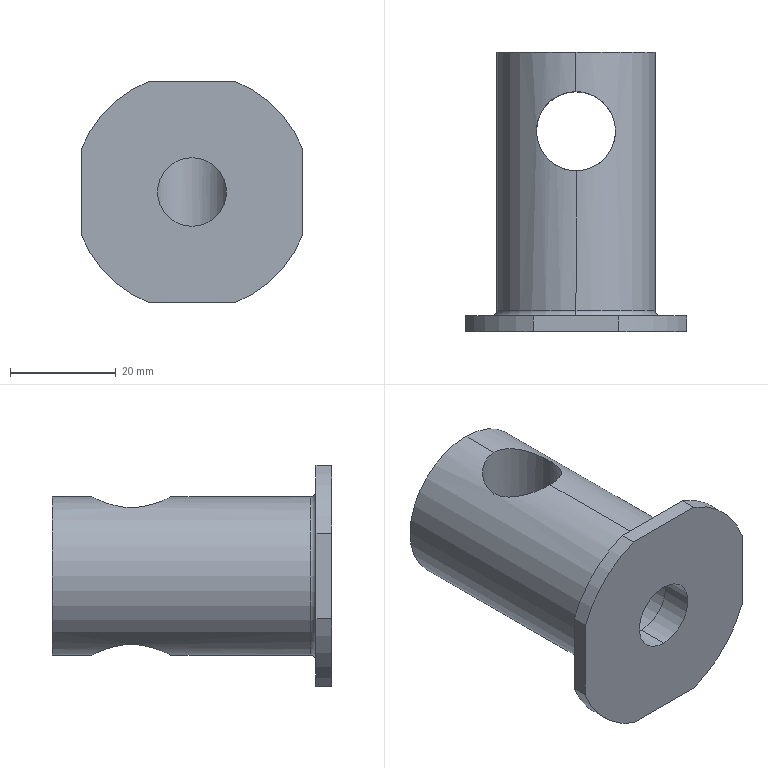Part | SolidWorks | features ICE 8, Fillet 2, MoveFace 1, Revolution 1 | 1 solid | 22 faces | box 42 x 53 x 42 mm | volume 30095 mm3 | cylinder 12 | plane 8 | torus 2 | commonest cylinder face diameters 45 x4 13 x2 14 x2 15 x2 30 x2
STEP:
#1=CARTESIAN_POINT('',(0.,31.,7.));
#2=VERTEX_POINT('',#1);
#3=CARTESIAN_POINT('',(0.,31.,-7.));
#4=VERTEX_POINT('',#3);
#5=CARTESIAN_POINT('',(0.,31.,7.));
#6=CARTESIAN_POINT('',(0.5148,31.,7.));
#7=CARTESIAN_POINT('',(1.015,31.052,6.944));
#8=CARTESIAN_POINT('',(1.746,31.202,6.783));
#9=CARTESIAN_POINT('',(1.988,31.264,6.716));
#10=CARTESIAN_POINT('',(2.452,31.408,6.561));
#11=CARTESIAN_POINT('',(2.676,31.49,6.473));
#12=CARTESIAN_POINT('',(3.325,31.761,6.178));
#13=CARTESIAN_POINT('',(3.73,31.979,5.941));
#14=CARTESIAN_POINT('',(4.457,32.452,5.416));
#15=CARTESIAN_POINT('',(4.784,32.71,5.128));
#16=CARTESIAN_POINT('',(5.228,33.118,4.66));
#17=CARTESIAN_POINT('',(5.368,33.259,4.498));
#18=CARTESIAN_POINT('',(5.63,33.541,4.165));
#19=CARTESIAN_POINT('',(5.752,33.684,3.994));
#20=CARTESIAN_POINT('',(6.094,34.112,3.47));
#21=CARTESIAN_POINT('',(6.288,34.4,3.104));
#22=CARTESIAN_POINT('',(6.617,34.955,2.322));
#23=CARTESIAN_POINT('',(6.752,35.227,1.904));
#24=CARTESIAN_POINT('',(6.896,35.549,1.224));
#25=CARTESIAN_POINT('',(6.935,35.643,0.9854));
#26=CARTESIAN_POINT('',(6.974,35.74,0.6181));
#27=CARTESIAN_POINT('',(6.984,35.765,0.494));
#28=CARTESIAN_POINT('',(6.997,35.8,0.2415));
#29=CARTESIAN_POINT('',(7.,35.808,0.112));
#30=CARTESIAN_POINT('',(6.999,35.806,-0.2717));
#31=CARTESIAN_POINT('',(6.985,35.767,-0.5222));
#32=CARTESIAN_POINT('',(6.93,35.632,-1.015));
#33=CARTESIAN_POINT('',(6.891,35.538,-1.249));
#34=CARTESIAN_POINT('',(6.795,35.323,-1.699));
#35=CARTESIAN_POINT('',(6.737,35.2,-1.915));
#36=CARTESIAN_POINT('',(6.603,34.94,-2.334));
#37=CARTESIAN_POINT('',(6.528,34.804,-2.535));
#38=CARTESIAN_POINT('',(6.28,34.388,-3.12));
#39=CARTESIAN_POINT('',(6.085,34.1,-3.486));
#40=CARTESIAN_POINT('',(5.626,33.527,-4.186));
#41=CARTESIAN_POINT('',(5.362,33.241,-4.52));
#42=CARTESIAN_POINT('',(4.774,32.702,-5.138));
#43=CARTESIAN_POINT('',(4.449,32.446,-5.423));
#44=CARTESIAN_POINT('',(3.905,32.093,-5.814));
#45=CARTESIAN_POINT('',(3.715,31.981,-5.937));
#46=CARTESIAN_POINT('',(3.313,31.767,-6.171));
#47=CARTESIAN_POINT('',(3.103,31.668,-6.279));
#48=CARTESIAN_POINT('',(2.671,31.488,-6.475));
#49=CARTESIAN_POINT('',(2.447,31.406,-6.563));
#50=CARTESIAN_POINT('',(1.985,31.263,-6.717));
#51=CARTESIAN_POINT('',(1.744,31.201,-6.784));
#52=CARTESIAN_POINT('',(1.01,31.051,-6.945));
#53=CARTESIAN_POINT('',(0.5101,31.,-7.));
#54=CARTESIAN_POINT('',(0.,31.,-7.));
#55=B_SPLINE_CURVE_WITH_KNOTS('',3,(#5,#6,#7,#8,#9,#10,#11,#12,#13,#14,#15,#16,#17,#18,#19,#20,#21,#22,#23,#24,#25,#26,#27,#28,#29,#30,#31,#32,#33,#34,#35,#36,#37,#38,#39,#40,#41,#42,#43,#44,#45,#46,#47,#48,#49,#50,#51,#52,#53,#54),.UNSPECIFIED.,.F.,.F.,(4,2,2,2,2,2,2,2,2,2,2,2,2,2,2,2,2,2,2,2,2,2,2,2,4),(0.,0.001518,0.002277,0.003036,0.004554,0.006073,0.006832,0.007591,0.009109,0.01063,0.01139,0.01177,0.01215,0.0129,0.01366,0.01442,0.01518,0.0167,0.01822,0.01974,0.02049,0.02125,0.02201,0.02277,0.02429),.UNSPECIFIED.);
#56=EDGE_CURVE('',#2,#4,#55,.T.);
#57=ORIENTED_EDGE('',*,*,#56,.F.);
#58=CARTESIAN_POINT('',(0.,31.,-7.));
#59=CARTESIAN_POINT('',(-0.2549,31.,-7.));
#60=CARTESIAN_POINT('',(-0.5127,31.013,-6.986));
#61=CARTESIAN_POINT('',(-1.015,31.065,-6.931));
#62=CARTESIAN_POINT('',(-1.263,31.103,-6.89));
#63=CARTESIAN_POINT('',(-1.75,31.203,-6.782));
#64=CARTESIAN_POINT('',(-1.991,31.265,-6.715));
#65=CARTESIAN_POINT('',(-2.455,31.409,-6.56));
#66=CARTESIAN_POINT('',(-2.679,31.491,-6.471));
#67=CARTESIAN_POINT('',(-3.328,31.763,-6.177));
#68=CARTESIAN_POINT('',(-3.733,31.98,-5.939));
#69=CARTESIAN_POINT('',(-4.459,32.454,-5.414));
#70=CARTESIAN_POINT('',(-4.786,32.711,-5.127));
#71=CARTESIAN_POINT('',(-5.229,33.12,-4.659));
#72=CARTESIAN_POINT('',(-5.369,33.26,-4.496));
#73=CARTESIAN_POINT('',(-5.631,33.543,-4.163));
#74=CARTESIAN_POINT('',(-5.753,33.685,-3.993));
#75=CARTESIAN_POINT('',(-6.094,34.113,-3.469));
#76=CARTESIAN_POINT('',(-6.289,34.401,-3.103));
#77=CARTESIAN_POINT('',(-6.617,34.956,-2.321));
#78=CARTESIAN_POINT('',(-6.752,35.227,-1.903));
#79=CARTESIAN_POINT('',(-6.896,35.549,-1.224));
#80=CARTESIAN_POINT('',(-6.935,35.643,-0.9852));
#81=CARTESIAN_POINT('',(-6.974,35.74,-0.6182));
#82=CARTESIAN_POINT('',(-6.984,35.765,-0.4941));
#83=CARTESIAN_POINT('',(-6.997,35.799,-0.2417));
#84=CARTESIAN_POINT('',(-7.,35.808,-0.1122));
#85=CARTESIAN_POINT('',(-6.999,35.806,0.2711));
#86=CARTESIAN_POINT('',(-6.985,35.768,0.5215));
#87=CARTESIAN_POINT('',(-6.931,35.633,1.014));
#88=CARTESIAN_POINT('',(-6.892,35.539,1.248));
#89=CARTESIAN_POINT('',(-6.795,35.323,1.697));
#90=CARTESIAN_POINT('',(-6.737,35.201,1.914));
#91=CARTESIAN_POINT('',(-6.603,34.941,2.333));
#92=CARTESIAN_POINT('',(-6.529,34.805,2.534));
#93=CARTESIAN_POINT('',(-6.281,34.389,3.118));
#94=CARTESIAN_POINT('',(-6.086,34.101,3.484));
#95=CARTESIAN_POINT('',(-5.628,33.529,4.184));
#96=CARTESIAN_POINT('',(-5.364,33.243,4.518));
#97=CARTESIAN_POINT('',(-4.776,32.704,5.135));
#98=CARTESIAN_POINT('',(-4.452,32.449,5.421));
#99=CARTESIAN_POINT('',(-3.909,32.096,5.811));
#100=CARTESIAN_POINT('',(-3.719,31.983,5.935));
#101=CARTESIAN_POINT('',(-3.317,31.769,6.169));
#102=CARTESIAN_POINT('',(-3.107,31.67,6.277));
#103=CARTESIAN_POINT('',(-2.675,31.49,6.473));
#104=CARTESIAN_POINT('',(-2.452,31.408,6.561));
#105=CARTESIAN_POINT('',(-1.99,31.265,6.716));
#106=CARTESIAN_POINT('',(-1.749,31.203,6.783));
#107=CARTESIAN_POINT('',(-1.015,31.052,6.944));
#108=CARTESIAN_POINT('',(-0.5145,31.,7.));
#109=CARTESIAN_POINT('',(0.,31.,7.));
#110=B_SPLINE_CURVE_WITH_KNOTS('',3,(#58,#59,#60,#61,#62,#63,#64,#65,#66,#67,#68,#69,#70,#71,#72,#73,#74,#75,#76,#77,#78,#79,#80,#81,#82,#83,#84,#85,#86,#87,#88,#89,#90,#91,#92,#93,#94,#95,#96,#97,#98,#99,#100,#101,#102,#103,#104,#105,#106,#107,#108,#109),.UNSPECIFIED.,.F.,.F.,(4,2,2,2,2,2,2,2,2,2,2,2,2,2,2,2,2,2,2,2,2,2,2,2,2,4),(0.02429,0.02505,0.02581,0.02657,0.02732,0.02884,0.03036,0.03112,0.03188,0.03339,0.03491,0.03567,0.03605,0.03643,0.03719,0.03795,0.0387,0.03946,0.04098,0.0425,0.04401,0.04477,0.04553,0.04629,0.04705,0.04857),.UNSPECIFIED.);
#111=EDGE_CURVE('',#4,#2,#110,.T.);
#112=ORIENTED_EDGE('',*,*,#111,.F.);
#113=EDGE_LOOP('',(#57,#112));
#114=FACE_BOUND('',#113,.T.);
#115=CARTESIAN_POINT('',(0.,31.,-15.));
#116=VERTEX_POINT('',#115);
#117=CARTESIAN_POINT('',(-7.5,38.5,-12.99));
#118=VERTEX_POINT('',#117);
#119=CARTESIAN_POINT('',(0.,31.,-15.));
#120=CARTESIAN_POINT('',(-0.2495,31.,-15.));
#121=CARTESIAN_POINT('',(-0.5024,31.013,-14.994));
#122=CARTESIAN_POINT('',(-1.,31.063,-14.969));
#123=CARTESIAN_POINT('',(-1.246,31.1,-14.95));
#124=CARTESIAN_POINT('',(-1.731,31.198,-14.902));
#125=CARTESIAN_POINT('',(-1.97,31.259,-14.872));
#126=CARTESIAN_POINT('',(-2.443,31.405,-14.802));
#127=CARTESIAN_POINT('',(-2.677,31.49,-14.761));
#128=CARTESIAN_POINT('',(-3.359,31.776,-14.626));
#129=CARTESIAN_POINT('',(-3.787,32.008,-14.52));
#130=CARTESIAN_POINT('',(-4.391,32.415,-14.345));
#131=CARTESIAN_POINT('',(-4.587,32.561,-14.283));
#132=CARTESIAN_POINT('',(-4.961,32.87,-14.157));
#133=CARTESIAN_POINT('',(-5.139,33.033,-14.093));
#134=CARTESIAN_POINT('',(-5.649,33.543,-13.9));
#135=CARTESIAN_POINT('',(-5.954,33.914,-13.771));
#136=CARTESIAN_POINT('',(-6.497,34.722,-13.523));
#137=CARTESIAN_POINT('',(-6.728,35.151,-13.408));
#138=CARTESIAN_POINT('',(-7.01,35.822,-13.262));
#139=CARTESIAN_POINT('',(-7.093,36.052,-13.217));
#140=CARTESIAN_POINT('',(-7.239,36.522,-13.138));
#141=CARTESIAN_POINT('',(-7.301,36.764,-13.104));
#142=CARTESIAN_POINT('',(-7.45,37.499,-13.02));
#143=CARTESIAN_POINT('',(-7.5,37.995,-12.99));
#144=CARTESIAN_POINT('',(-7.5,38.5,-12.99));
#145=B_SPLINE_CURVE_WITH_KNOTS('',3,(#119,#120,#121,#122,#123,#124,#125,#126,#127,#128,#129,#130,#131,#132,#133,#134,#135,#136,#137,#138,#139,#140,#141,#142,#143,#144),.UNSPECIFIED.,.F.,.F.,(4,2,2,2,2,2,2,2,2,2,2,2,4),(0.01193,0.01268,0.01342,0.01417,0.01491,0.0164,0.01714,0.01789,0.01938,0.02086,0.02161,0.02235,0.02384),.UNSPECIFIED.);
#146=EDGE_CURVE('',#116,#118,#145,.T.);
#147=ORIENTED_EDGE('',*,*,#146,.T.);
#148=CARTESIAN_POINT('',(-7.5,38.5,12.99));
#149=VERTEX_POINT('',#148);
#150=CARTESIAN_POINT('',(-7.5,38.5,-15.));
#151=DIRECTION('',(0.,0.,1.));
#152=VECTOR('',#151,1000.);
#153=LINE('',#150,#152);
#154=EDGE_CURVE('',#118,#149,#153,.T.);
#155=ORIENTED_EDGE('',*,*,#154,.T.);
#156=CARTESIAN_POINT('',(0.,31.,15.));
#157=VERTEX_POINT('',#156);
#158=CARTESIAN_POINT('',(-7.5,38.5,12.99));
#159=CARTESIAN_POINT('',(-7.5,37.995,12.99));
#160=CARTESIAN_POINT('',(-7.45,37.5,13.02));
#161=CARTESIAN_POINT('',(-7.254,36.53,13.13));
#162=CARTESIAN_POINT('',(-7.106,36.05,13.212));
#163=CARTESIAN_POINT('',(-6.727,35.147,13.409));
#164=CARTESIAN_POINT('',(-6.496,34.72,13.524));
#165=CARTESIAN_POINT('',(-6.089,34.114,13.71));
#166=CARTESIAN_POINT('',(-5.943,33.918,13.774));
#167=CARTESIAN_POINT('',(-5.636,33.545,13.902));
#168=CARTESIAN_POINT('',(-5.474,33.367,13.967));
#169=CARTESIAN_POINT('',(-5.134,33.027,14.095));
#170=CARTESIAN_POINT('',(-4.955,32.865,14.159));
#171=CARTESIAN_POINT('',(-4.581,32.557,14.285));
#172=CARTESIAN_POINT('',(-4.385,32.41,14.346));
#173=CARTESIAN_POINT('',(-3.778,32.003,14.523));
#174=CARTESIAN_POINT('',(-3.351,31.772,14.628));
#175=CARTESIAN_POINT('',(-2.674,31.489,14.761));
#176=CARTESIAN_POINT('',(-2.443,31.405,14.802));
#177=CARTESIAN_POINT('',(-1.967,31.258,14.872));
#178=CARTESIAN_POINT('',(-1.724,31.197,14.903));
#179=CARTESIAN_POINT('',(-0.9934,31.05,14.975));
#180=CARTESIAN_POINT('',(-0.5001,31.,15.));
#181=CARTESIAN_POINT('',(0.,31.,15.));
#182=B_SPLINE_CURVE_WITH_KNOTS('',3,(#158,#159,#160,#161,#162,#163,#164,#165,#166,#167,#168,#169,#170,#171,#172,#173,#174,#175,#176,#177,#178,#179,#180,#181),.UNSPECIFIED.,.F.,.F.,(4,2,2,2,2,2,2,2,2,2,2,4),(0.,0.001492,0.002983,0.004475,0.00522,0.005966,0.006712,0.007458,0.008949,0.009695,0.01044,0.01193),.UNSPECIFIED.);
#183=EDGE_CURVE('',#149,#157,#182,.T.);
#184=ORIENTED_EDGE('',*,*,#183,.T.);
#185=CARTESIAN_POINT('',(7.5,38.5,12.99));
#186=VERTEX_POINT('',#185);
#187=CARTESIAN_POINT('',(0.,31.,15.));
#188=CARTESIAN_POINT('',(0.2495,31.,15.));
#189=CARTESIAN_POINT('',(0.5024,31.013,14.994));
#190=CARTESIAN_POINT('',(1.,31.063,14.969));
#191=CARTESIAN_POINT('',(1.246,31.1,14.95));
#192=CARTESIAN_POINT('',(1.731,31.198,14.902));
#193=CARTESIAN_POINT('',(1.97,31.259,14.872));
#194=CARTESIAN_POINT('',(2.443,31.405,14.802));
#195=CARTESIAN_POINT('',(2.677,31.49,14.761));
#196=CARTESIAN_POINT('',(3.359,31.776,14.626));
#197=CARTESIAN_POINT('',(3.787,32.008,14.52));
#198=CARTESIAN_POINT('',(4.391,32.415,14.345));
#199=CARTESIAN_POINT('',(4.587,32.561,14.283));
#200=CARTESIAN_POINT('',(4.961,32.87,14.157));
#201=CARTESIAN_POINT('',(5.139,33.033,14.093));
#202=CARTESIAN_POINT('',(5.649,33.543,13.9));
#203=CARTESIAN_POINT('',(5.954,33.914,13.771));
#204=CARTESIAN_POINT('',(6.497,34.722,13.523));
#205=CARTESIAN_POINT('',(6.728,35.151,13.408));
#206=CARTESIAN_POINT('',(7.01,35.822,13.262));
#207=CARTESIAN_POINT('',(7.093,36.052,13.217));
#208=CARTESIAN_POINT('',(7.239,36.522,13.138));
#209=CARTESIAN_POINT('',(7.301,36.764,13.104));
#210=CARTESIAN_POINT('',(7.45,37.499,13.02));
#211=CARTESIAN_POINT('',(7.5,37.995,12.99));
#212=CARTESIAN_POINT('',(7.5,38.5,12.99));
#213=B_SPLINE_CURVE_WITH_KNOTS('',3,(#187,#188,#189,#190,#191,#192,#193,#194,#195,#196,#197,#198,#199,#200,#201,#202,#203,#204,#205,#206,#207,#208,#209,#210,#211,#212),.UNSPECIFIED.,.F.,.F.,(4,2,2,2,2,2,2,2,2,2,2,2,4),(0.01193,0.01268,0.01342,0.01417,0.01491,0.0164,0.01714,0.01789,0.01938,0.02086,0.02161,0.02235,0.02384),.UNSPECIFIED.);
#214=EDGE_CURVE('',#157,#186,#213,.T.);
#215=ORIENTED_EDGE('',*,*,#214,.T.);
#216=CARTESIAN_POINT('',(7.5,38.5,-12.99));
#217=VERTEX_POINT('',#216);
#218=CARTESIAN_POINT('',(7.5,38.5,-15.));
#219=DIRECTION('',(0.,0.,1.));
#220=VECTOR('',#219,1000.);
#221=LINE('',#218,#220);
#222=EDGE_CURVE('',#217,#186,#221,.T.);
#223=ORIENTED_EDGE('',*,*,#222,.F.);
#224=CARTESIAN_POINT('',(7.5,38.5,-12.99));
#225=CARTESIAN_POINT('',(7.5,37.995,-12.99));
#226=CARTESIAN_POINT('',(7.45,37.5,-13.02));
#227=CARTESIAN_POINT('',(7.254,36.53,-13.13));
#228=CARTESIAN_POINT('',(7.106,36.05,-13.212));
#229=CARTESIAN_POINT('',(6.727,35.147,-13.409));
#230=CARTESIAN_POINT('',(6.496,34.72,-13.524));
#231=CARTESIAN_POINT('',(6.089,34.114,-13.71));
#232=CARTESIAN_POINT('',(5.943,33.918,-13.774));
#233=CARTESIAN_POINT('',(5.636,33.545,-13.902));
#234=CARTESIAN_POINT('',(5.474,33.367,-13.967));
#235=CARTESIAN_POINT('',(5.134,33.027,-14.095));
#236=CARTESIAN_POINT('',(4.955,32.865,-14.159));
#237=CARTESIAN_POINT('',(4.581,32.557,-14.285));
#238=CARTESIAN_POINT('',(4.385,32.41,-14.346));
#239=CARTESIAN_POINT('',(3.778,32.003,-14.523));
#240=CARTESIAN_POINT('',(3.351,31.772,-14.628));
#241=CARTESIAN_POINT('',(2.674,31.489,-14.761));
#242=CARTESIAN_POINT('',(2.443,31.405,-14.802));
#243=CARTESIAN_POINT('',(1.967,31.258,-14.872));
#244=CARTESIAN_POINT('',(1.724,31.197,-14.903));
#245=CARTESIAN_POINT('',(0.9934,31.05,-14.975));
#246=CARTESIAN_POINT('',(0.5001,31.,-15.));
#247=CARTESIAN_POINT('',(0.,31.,-15.));
#248=B_SPLINE_CURVE_WITH_KNOTS('',3,(#224,#225,#226,#227,#228,#229,#230,#231,#232,#233,#234,#235,#236,#237,#238,#239,#240,#241,#242,#243,#244,#245,#246,#247),.UNSPECIFIED.,.F.,.F.,(4,2,2,2,2,2,2,2,2,2,2,4),(0.,0.001492,0.002983,0.004475,0.00522,0.005966,0.006712,0.007458,0.008949,0.009695,0.01044,0.01193),.UNSPECIFIED.);
#249=EDGE_CURVE('',#217,#116,#248,.T.);
#250=ORIENTED_EDGE('',*,*,#249,.T.);
#251=EDGE_LOOP('',(#147,#155,#184,#215,#223,#250));
#252=FACE_OUTER_BOUND('',#251,.T.);
#253=CARTESIAN_POINT('',(0.,38.5,-15.));
#254=DIRECTION('',(0.,0.,1.));
#255=DIRECTION('',(1.,0.,0.));
#256=AXIS2_PLACEMENT_3D('',#253,#254,#255);
#257=CYLINDRICAL_SURFACE('',#256,7.5);
#258=ADVANCED_FACE('',(#114,#252),#257,.F.);
#259=CARTESIAN_POINT('',(0.,0.5,6.5));
#260=VERTEX_POINT('',#259);
#261=CARTESIAN_POINT('',(0.,0.5,-6.5));
#262=VERTEX_POINT('',#261);
#263=CARTESIAN_POINT('',(0.,0.5,0.));
#264=DIRECTION('',(0.,-1.,0.));
#265=DIRECTION('',(0.,0.,1.));
#266=AXIS2_PLACEMENT_3D('',#263,#264,#265);
#267=CIRCLE('',#266,6.5);
#268=EDGE_CURVE('',#260,#262,#267,.T.);
#269=ORIENTED_EDGE('',*,*,#268,.T.);
#270=CARTESIAN_POINT('',(0.,6.5,-6.5));
#271=VERTEX_POINT('',#270);
#272=CARTESIAN_POINT('',(0.,-23.5,-6.5));
#273=DIRECTION('',(0.,1.,0.));
#274=VECTOR('',#273,1000.);
#275=LINE('',#272,#274);
#276=EDGE_CURVE('',#262,#271,#275,.T.);
#277=ORIENTED_EDGE('',*,*,#276,.T.);
#278=CARTESIAN_POINT('',(0.,6.5,6.5));
#279=VERTEX_POINT('',#278);
#280=CARTESIAN_POINT('',(0.,6.5,0.));
#281=DIRECTION('',(0.,1.,0.));
#282=DIRECTION('',(0.,0.,1.));
#283=AXIS2_PLACEMENT_3D('',#280,#281,#282);
#284=CIRCLE('',#283,6.5);
#285=EDGE_CURVE('',#271,#279,#284,.T.);
#286=ORIENTED_EDGE('',*,*,#285,.T.);
#287=CARTESIAN_POINT('',(0.,-23.5,6.5));
#288=DIRECTION('',(0.,1.,0.));
#289=VECTOR('',#288,1000.);
#290=LINE('',#287,#289);
#291=EDGE_CURVE('',#260,#279,#290,.T.);
#292=ORIENTED_EDGE('',*,*,#291,.F.);
#293=EDGE_LOOP('',(#269,#277,#286,#292));
#294=FACE_OUTER_BOUND('',#293,.T.);
#295=CARTESIAN_POINT('',(0.,-23.5,0.));
#296=DIRECTION('',(0.,1.,0.));
#297=DIRECTION('',(0.,0.,1.));
#298=AXIS2_PLACEMENT_3D('',#295,#296,#297);
#299=CYLINDRICAL_SURFACE('',#298,6.5);
#300=ADVANCED_FACE('',(#294),#299,.F.);
#301=CARTESIAN_POINT('',(0.,6.5,-7.));
#302=VERTEX_POINT('',#301);
#303=CARTESIAN_POINT('',(0.,6.5,7.));
#304=VERTEX_POINT('',#303);
#305=CARTESIAN_POINT('',(0.,6.5,0.));
#306=DIRECTION('',(0.,1.,0.));
#307=DIRECTION('',(0.,0.,1.));
#308=AXIS2_PLACEMENT_3D('',#305,#306,#307);
#309=CIRCLE('',#308,7.);
#310=EDGE_CURVE('',#302,#304,#309,.T.);
#311=ORIENTED_EDGE('',*,*,#310,.F.);
#312=CARTESIAN_POINT('',(0.,26.5,-7.));
#313=DIRECTION('',(0.,1.,0.));
#314=VECTOR('',#313,1000.);
#315=LINE('',#312,#314);
#316=EDGE_CURVE('',#302,#4,#315,.T.);
#317=ORIENTED_EDGE('',*,*,#316,.T.);
#318=ORIENTED_EDGE('',*,*,#111,.T.);
#319=CARTESIAN_POINT('',(0.,26.5,7.));
#320=DIRECTION('',(0.,1.,0.));
#321=VECTOR('',#320,1000.);
#322=LINE('',#319,#321);
#323=EDGE_CURVE('',#304,#2,#322,.T.);
#324=ORIENTED_EDGE('',*,*,#323,.F.);
#325=EDGE_LOOP('',(#311,#317,#318,#324));
#326=FACE_OUTER_BOUND('',#325,.T.);
#327=CARTESIAN_POINT('',(0.,26.5,0.));
#328=DIRECTION('',(0.,1.,0.));
#329=DIRECTION('',(0.,0.,1.));
#330=AXIS2_PLACEMENT_3D('',#327,#328,#329);
#331=CYLINDRICAL_SURFACE('',#330,7.);
#332=ADVANCED_FACE('',(#326),#331,.F.);
#333=CARTESIAN_POINT('',(0.,4.5,-15.));
#334=VERTEX_POINT('',#333);
#335=CARTESIAN_POINT('',(0.,4.5,15.));
#336=VERTEX_POINT('',#335);
#337=CARTESIAN_POINT('',(0.,4.5,0.));
#338=DIRECTION('',(0.,1.,0.));
#339=DIRECTION('',(0.,0.,1.));
#340=AXIS2_PLACEMENT_3D('',#337,#338,#339);
#341=CIRCLE('',#340,15.);
#342=EDGE_CURVE('',#334,#336,#341,.T.);
#343=ORIENTED_EDGE('',*,*,#342,.F.);
#344=CARTESIAN_POINT('',(0.,3.5,-16.));
#345=VERTEX_POINT('',#344);
#346=CARTESIAN_POINT('',(0.,4.5,-16.));
#347=DIRECTION('',(1.,0.,0.));
#348=DIRECTION('',(0.,0.,-1.));
#349=AXIS2_PLACEMENT_3D('',#346,#347,#348);
#350=CIRCLE('',#349,1.);
#351=EDGE_CURVE('',#334,#345,#350,.T.);
#352=ORIENTED_EDGE('',*,*,#351,.T.);
#353=CARTESIAN_POINT('',(0.,3.5,16.));
#354=VERTEX_POINT('',#353);
#355=CARTESIAN_POINT('',(0.,3.5,0.));
#356=DIRECTION('',(0.,-1.,0.));
#357=DIRECTION('',(0.,0.,1.));
#358=AXIS2_PLACEMENT_3D('',#355,#356,#357);
#359=CIRCLE('',#358,16.);
#360=EDGE_CURVE('',#354,#345,#359,.T.);
#361=ORIENTED_EDGE('',*,*,#360,.F.);
#362=CARTESIAN_POINT('',(0.,4.5,16.));
#363=DIRECTION('',(-1.,0.,0.));
#364=DIRECTION('',(0.,0.,1.));
#365=AXIS2_PLACEMENT_3D('',#362,#363,#364);
#366=CIRCLE('',#365,1.);
#367=EDGE_CURVE('',#336,#354,#366,.T.);
#368=ORIENTED_EDGE('',*,*,#367,.F.);
#369=EDGE_LOOP('',(#343,#352,#361,#368));
#370=FACE_OUTER_BOUND('',#369,.T.);
#371=CARTESIAN_POINT('',(0.,4.5,0.));
#372=DIRECTION('',(0.,1.,0.));
#373=DIRECTION('',(0.,0.,1.));
#374=AXIS2_PLACEMENT_3D('',#371,#372,#373);
#375=TOROIDAL_SURFACE('',#374,16.,1.);
#376=ADVANCED_FACE('',(#370),#375,.F.);
#377=CARTESIAN_POINT('',(0.,4.5,0.));
#378=DIRECTION('',(0.,1.,0.));
#379=DIRECTION('',(0.,0.,1.));
#380=AXIS2_PLACEMENT_3D('',#377,#378,#379);
#381=CIRCLE('',#380,15.);
#382=EDGE_CURVE('',#336,#334,#381,.T.);
#383=ORIENTED_EDGE('',*,*,#382,.T.);
#384=CARTESIAN_POINT('',(0.,38.5,-15.));
#385=DIRECTION('',(0.,1.,0.));
#386=VECTOR('',#385,1000.);
#387=LINE('',#384,#386);
#388=EDGE_CURVE('',#334,#116,#387,.T.);
#389=ORIENTED_EDGE('',*,*,#388,.T.);
#390=ORIENTED_EDGE('',*,*,#249,.F.);
#391=CARTESIAN_POINT('',(0.,46.,-15.));
#392=VERTEX_POINT('',#391);
#393=CARTESIAN_POINT('',(0.,46.,-15.));
#394=CARTESIAN_POINT('',(0.2481,46.,-15.));
#395=CARTESIAN_POINT('',(0.4965,45.988,-14.994));
#396=CARTESIAN_POINT('',(0.9939,45.938,-14.969));
#397=CARTESIAN_POINT('',(1.244,45.9,-14.95));
#398=CARTESIAN_POINT('',(1.976,45.752,-14.877));
#399=CARTESIAN_POINT('',(2.446,45.607,-14.806));
#400=CARTESIAN_POINT('',(3.128,45.321,-14.672));
#401=CARTESIAN_POINT('',(3.351,45.214,-14.623));
#402=CARTESIAN_POINT('',(3.782,44.981,-14.517));
#403=CARTESIAN_POINT('',(3.989,44.856,-14.461));
#404=CARTESIAN_POINT('',(4.391,44.585,-14.344));
#405=CARTESIAN_POINT('',(4.584,44.441,-14.284));
#406=CARTESIAN_POINT('',(4.958,44.133,-14.158));
#407=CARTESIAN_POINT('',(5.139,43.968,-14.094));
#408=CARTESIAN_POINT('',(5.651,43.454,-13.899));
#409=CARTESIAN_POINT('',(5.956,43.083,-13.77));
#410=CARTESIAN_POINT('',(6.494,42.283,-13.525));
#411=CARTESIAN_POINT('',(6.729,41.848,-13.408));
#412=CARTESIAN_POINT('',(7.106,40.948,-13.212));
#413=CARTESIAN_POINT('',(7.251,40.481,-13.132));
#414=CARTESIAN_POINT('',(7.448,39.51,-13.021));
#415=CARTESIAN_POINT('',(7.5,39.004,-12.99));
#416=CARTESIAN_POINT('',(7.5,38.5,-12.99));
#417=B_SPLINE_CURVE_WITH_KNOTS('',3,(#393,#394,#395,#396,#397,#398,#399,#400,#401,#402,#403,#404,#405,#406,#407,#408,#409,#410,#411,#412,#413,#414,#415,#416),.UNSPECIFIED.,.F.,.F.,(4,2,2,2,2,2,2,2,2,2,2,4),(0.03575,0.03649,0.03724,0.03873,0.03947,0.04021,0.04096,0.0417,0.04319,0.04468,0.04616,0.04765),.UNSPECIFIED.);
#418=EDGE_CURVE('',#392,#217,#417,.T.);
#419=ORIENTED_EDGE('',*,*,#418,.F.);
#420=CARTESIAN_POINT('',(0.,53.5,-15.));
#421=VERTEX_POINT('',#420);
#422=CARTESIAN_POINT('',(0.,38.5,-15.));
#423=DIRECTION('',(0.,1.,0.));
#424=VECTOR('',#423,1000.);
#425=LINE('',#422,#424);
#426=EDGE_CURVE('',#392,#421,#425,.T.);
#427=ORIENTED_EDGE('',*,*,#426,.T.);
#428=CARTESIAN_POINT('',(0.,53.5,15.));
#429=VERTEX_POINT('',#428);
#430=CARTESIAN_POINT('',(0.,53.5,0.));
#431=DIRECTION('',(0.,1.,0.));
#432=DIRECTION('',(0.,0.,1.));
#433=AXIS2_PLACEMENT_3D('',#430,#431,#432);
#434=CIRCLE('',#433,15.);
#435=EDGE_CURVE('',#429,#421,#434,.T.);
#436=ORIENTED_EDGE('',*,*,#435,.F.);
#437=CARTESIAN_POINT('',(0.,46.,15.));
#438=VERTEX_POINT('',#437);
#439=CARTESIAN_POINT('',(0.,38.5,15.));
#440=DIRECTION('',(0.,1.,0.));
#441=VECTOR('',#440,1000.);
#442=LINE('',#439,#441);
#443=EDGE_CURVE('',#438,#429,#442,.T.);
#444=ORIENTED_EDGE('',*,*,#443,.F.);
#445=CARTESIAN_POINT('',(7.5,38.5,12.99));
#446=CARTESIAN_POINT('',(7.5,38.752,12.99));
#447=CARTESIAN_POINT('',(7.487,39.005,12.998));
#448=CARTESIAN_POINT('',(7.437,39.503,13.027));
#449=CARTESIAN_POINT('',(7.399,39.749,13.048));
#450=CARTESIAN_POINT('',(7.301,40.234,13.103));
#451=CARTESIAN_POINT('',(7.24,40.473,13.137));
#452=CARTESIAN_POINT('',(7.095,40.945,13.216));
#453=CARTESIAN_POINT('',(7.01,41.179,13.262));
#454=CARTESIAN_POINT('',(6.724,41.859,13.41));
#455=CARTESIAN_POINT('',(6.493,42.285,13.525));
#456=CARTESIAN_POINT('',(6.087,42.888,13.71));
#457=CARTESIAN_POINT('',(5.941,43.084,13.774));
#458=CARTESIAN_POINT('',(5.633,43.458,13.903));
#459=CARTESIAN_POINT('',(5.47,43.636,13.968));
#460=CARTESIAN_POINT('',(4.96,44.146,14.161));
#461=CARTESIAN_POINT('',(4.589,44.453,14.287));
#462=CARTESIAN_POINT('',(3.776,44.998,14.523));
#463=CARTESIAN_POINT('',(3.347,45.23,14.629));
#464=CARTESIAN_POINT('',(2.672,45.512,14.762));
#465=CARTESIAN_POINT('',(2.441,45.596,14.802));
#466=CARTESIAN_POINT('',(1.969,45.741,14.872));
#467=CARTESIAN_POINT('',(1.726,45.803,14.902));
#468=CARTESIAN_POINT('',(0.9912,45.951,14.975));
#469=CARTESIAN_POINT('',(0.4976,46.,15.));
#470=CARTESIAN_POINT('',(0.,46.,15.));
#471=B_SPLINE_CURVE_WITH_KNOTS('',3,(#445,#446,#447,#448,#449,#450,#451,#452,#453,#454,#455,#456,#457,#458,#459,#460,#461,#462,#463,#464,#465,#466,#467,#468,#469,#470),.UNSPECIFIED.,.F.,.F.,(4,2,2,2,2,2,2,2,2,2,2,2,4),(0.02384,0.02459,0.02533,0.02608,0.02682,0.02831,0.02905,0.0298,0.03129,0.03278,0.03352,0.03427,0.03575),.UNSPECIFIED.);
#472=EDGE_CURVE('',#186,#438,#471,.T.);
#473=ORIENTED_EDGE('',*,*,#472,.F.);
#474=ORIENTED_EDGE('',*,*,#214,.F.);
#475=CARTESIAN_POINT('',(0.,38.5,15.));
#476=DIRECTION('',(0.,1.,0.));
#477=VECTOR('',#476,1000.);
#478=LINE('',#475,#477);
#479=EDGE_CURVE('',#336,#157,#478,.T.);
#480=ORIENTED_EDGE('',*,*,#479,.F.);
#481=EDGE_LOOP('',(#383,#389,#390,#419,#427,#436,#444,#473,#474,#480));
#482=FACE_OUTER_BOUND('',#481,.T.);
#483=CARTESIAN_POINT('',(0.,38.5,0.));
#484=DIRECTION('',(0.,1.,0.));
#485=DIRECTION('',(0.,0.,1.));
#486=AXIS2_PLACEMENT_3D('',#483,#484,#485);
#487=CYLINDRICAL_SURFACE('',#486,15.);
#488=ADVANCED_FACE('',(#482),#487,.T.);
#489=CARTESIAN_POINT('',(-21.,0.5,8.078));
#490=VERTEX_POINT('',#489);
#491=CARTESIAN_POINT('',(-21.,0.5,-8.078));
#492=VERTEX_POINT('',#491);
#493=CARTESIAN_POINT('',(-21.,0.5,0.));
#494=DIRECTION('',(0.,0.,-1.));
#495=VECTOR('',#494,1000.);
#496=LINE('',#493,#495);
#497=EDGE_CURVE('',#490,#492,#496,.T.);
#498=ORIENTED_EDGE('',*,*,#497,.T.);
#499=CARTESIAN_POINT('',(-8.078,0.5,-21.));
#500=VERTEX_POINT('',#499);
#501=CARTESIAN_POINT('',(0.,0.5,0.));
#502=DIRECTION('',(0.,1.,0.));
#503=DIRECTION('',(0.,0.,1.));
#504=AXIS2_PLACEMENT_3D('',#501,#502,#503);
#505=CIRCLE('',#504,22.5);
#506=EDGE_CURVE('',#500,#492,#505,.T.);
#507=ORIENTED_EDGE('',*,*,#506,.F.);
#508=CARTESIAN_POINT('',(8.078,0.5,-21.));
#509=VERTEX_POINT('',#508);
#510=CARTESIAN_POINT('',(-22.5,0.5,-21.));
#511=DIRECTION('',(1.,0.,0.));
#512=VECTOR('',#511,1000.);
#513=LINE('',#510,#512);
#514=EDGE_CURVE('',#500,#509,#513,.T.);
#515=ORIENTED_EDGE('',*,*,#514,.T.);
#516=CARTESIAN_POINT('',(21.,0.5,-8.078));
#517=VERTEX_POINT('',#516);
#518=CARTESIAN_POINT('',(0.,0.5,0.));
#519=DIRECTION('',(0.,1.,0.));
#520=DIRECTION('',(0.,0.,1.));
#521=AXIS2_PLACEMENT_3D('',#518,#519,#520);
#522=CIRCLE('',#521,22.5);
#523=EDGE_CURVE('',#517,#509,#522,.T.);
#524=ORIENTED_EDGE('',*,*,#523,.F.);
#525=CARTESIAN_POINT('',(21.,0.5,8.078));
#526=VERTEX_POINT('',#525);
#527=CARTESIAN_POINT('',(21.,0.5,0.));
#528=DIRECTION('',(0.,0.,1.));
#529=VECTOR('',#528,1000.);
#530=LINE('',#527,#529);
#531=EDGE_CURVE('',#517,#526,#530,.T.);
#532=ORIENTED_EDGE('',*,*,#531,.T.);
#533=CARTESIAN_POINT('',(8.078,0.5,21.));
#534=VERTEX_POINT('',#533);
#535=CARTESIAN_POINT('',(0.,0.5,0.));
#536=DIRECTION('',(0.,1.,0.));
#537=DIRECTION('',(0.,0.,1.));
#538=AXIS2_PLACEMENT_3D('',#535,#536,#537);
#539=CIRCLE('',#538,22.5);
#540=EDGE_CURVE('',#534,#526,#539,.T.);
#541=ORIENTED_EDGE('',*,*,#540,.F.);
#542=CARTESIAN_POINT('',(-8.078,0.5,21.));
#543=VERTEX_POINT('',#542);
#544=CARTESIAN_POINT('',(-22.5,0.5,21.));
#545=DIRECTION('',(-1.,0.,0.));
#546=VECTOR('',#545,1000.);
#547=LINE('',#544,#546);
#548=EDGE_CURVE('',#534,#543,#547,.T.);
#549=ORIENTED_EDGE('',*,*,#548,.T.);
#550=CARTESIAN_POINT('',(0.,0.5,0.));
#551=DIRECTION('',(0.,1.,0.));
#552=DIRECTION('',(0.,0.,1.));
#553=AXIS2_PLACEMENT_3D('',#550,#551,#552);
#554=CIRCLE('',#553,22.5);
#555=EDGE_CURVE('',#490,#543,#554,.T.);
#556=ORIENTED_EDGE('',*,*,#555,.F.);
#557=EDGE_LOOP('',(#498,#507,#515,#524,#532,#541,#549,#556));
#558=FACE_OUTER_BOUND('',#557,.T.);
#559=ORIENTED_EDGE('',*,*,#268,.F.);
#560=CARTESIAN_POINT('',(0.,0.5,0.));
#561=DIRECTION('',(0.,-1.,0.));
#562=DIRECTION('',(0.,0.,1.));
#563=AXIS2_PLACEMENT_3D('',#560,#561,#562);
#564=CIRCLE('',#563,6.5);
#565=EDGE_CURVE('',#262,#260,#564,.T.);
#566=ORIENTED_EDGE('',*,*,#565,.F.);
#567=EDGE_LOOP('',(#559,#566));
#568=FACE_BOUND('',#567,.T.);
#569=CARTESIAN_POINT('',(-22.5,0.5,0.));
#570=DIRECTION('',(0.,-1.,0.));
#571=DIRECTION('',(0.,0.,-1.));
#572=AXIS2_PLACEMENT_3D('',#569,#570,#571);
#573=PLANE('',#572);
#574=ADVANCED_FACE('',(#558,#568),#573,.T.);
#575=CARTESIAN_POINT('',(-21.,3.5,8.078));
#576=VERTEX_POINT('',#575);
#577=CARTESIAN_POINT('',(-8.078,3.5,21.));
#578=VERTEX_POINT('',#577);
#579=CARTESIAN_POINT('',(0.,3.5,0.));
#580=DIRECTION('',(0.,1.,0.));
#581=DIRECTION('',(0.,0.,1.));
#582=AXIS2_PLACEMENT_3D('',#579,#580,#581);
#583=CIRCLE('',#582,22.5);
#584=EDGE_CURVE('',#576,#578,#583,.T.);
#585=ORIENTED_EDGE('',*,*,#584,.F.);
#586=CARTESIAN_POINT('',(-21.,18.5,8.078));
#587=DIRECTION('',(0.,-1.,0.));
#588=VECTOR('',#587,1000.);
#589=LINE('',#586,#588);
#590=EDGE_CURVE('',#576,#490,#589,.T.);
#591=ORIENTED_EDGE('',*,*,#590,.T.);
#592=ORIENTED_EDGE('',*,*,#555,.T.);
#593=CARTESIAN_POINT('',(-8.078,18.5,21.));
#594=DIRECTION('',(0.,1.,0.));
#595=VECTOR('',#594,1000.);
#596=LINE('',#593,#595);
#597=EDGE_CURVE('',#543,#578,#596,.T.);
#598=ORIENTED_EDGE('',*,*,#597,.T.);
#599=EDGE_LOOP('',(#585,#591,#592,#598));
#600=FACE_OUTER_BOUND('',#599,.T.);
#601=CARTESIAN_POINT('',(0.,18.5,0.));
#602=DIRECTION('',(0.,1.,0.));
#603=DIRECTION('',(0.,0.,1.));
#604=AXIS2_PLACEMENT_3D('',#601,#602,#603);
#605=CYLINDRICAL_SURFACE('',#604,22.5);
#606=ADVANCED_FACE('',(#600),#605,.T.);
#607=ORIENTED_EDGE('',*,*,#506,.T.);
#608=CARTESIAN_POINT('',(-21.,3.5,-8.078));
#609=VERTEX_POINT('',#608);
#610=CARTESIAN_POINT('',(-21.,18.5,-8.078));
#611=DIRECTION('',(0.,1.,0.));
#612=VECTOR('',#611,1000.);
#613=LINE('',#610,#612);
#614=EDGE_CURVE('',#492,#609,#613,.T.);
#615=ORIENTED_EDGE('',*,*,#614,.T.);
#616=CARTESIAN_POINT('',(-8.078,3.5,-21.));
#617=VERTEX_POINT('',#616);
#618=CARTESIAN_POINT('',(0.,3.5,0.));
#619=DIRECTION('',(0.,1.,0.));
#620=DIRECTION('',(0.,0.,1.));
#621=AXIS2_PLACEMENT_3D('',#618,#619,#620);
#622=CIRCLE('',#621,22.5);
#623=EDGE_CURVE('',#617,#609,#622,.T.);
#624=ORIENTED_EDGE('',*,*,#623,.F.);
#625=CARTESIAN_POINT('',(-8.078,18.5,-21.));
#626=DIRECTION('',(0.,-1.,0.));
#627=VECTOR('',#626,1000.);
#628=LINE('',#625,#627);
#629=EDGE_CURVE('',#617,#500,#628,.T.);
#630=ORIENTED_EDGE('',*,*,#629,.T.);
#631=EDGE_LOOP('',(#607,#615,#624,#630));
#632=FACE_OUTER_BOUND('',#631,.T.);
#633=CARTESIAN_POINT('',(0.,18.5,0.));
#634=DIRECTION('',(0.,1.,0.));
#635=DIRECTION('',(0.,0.,1.));
#636=AXIS2_PLACEMENT_3D('',#633,#634,#635);
#637=CYLINDRICAL_SURFACE('',#636,22.5);
#638=ADVANCED_FACE('',(#632),#637,.T.);
#639=ORIENTED_EDGE('',*,*,#523,.T.);
#640=CARTESIAN_POINT('',(8.078,3.5,-21.));
#641=VERTEX_POINT('',#640);
#642=CARTESIAN_POINT('',(8.078,18.5,-21.));
#643=DIRECTION('',(0.,1.,0.));
#644=VECTOR('',#643,1000.);
#645=LINE('',#642,#644);
#646=EDGE_CURVE('',#509,#641,#645,.T.);
#647=ORIENTED_EDGE('',*,*,#646,.T.);
#648=CARTESIAN_POINT('',(21.,3.5,-8.078));
#649=VERTEX_POINT('',#648);
#650=CARTESIAN_POINT('',(0.,3.5,0.));
#651=DIRECTION('',(0.,1.,0.));
#652=DIRECTION('',(0.,0.,1.));
#653=AXIS2_PLACEMENT_3D('',#650,#651,#652);
#654=CIRCLE('',#653,22.5);
#655=EDGE_CURVE('',#649,#641,#654,.T.);
#656=ORIENTED_EDGE('',*,*,#655,.F.);
#657=CARTESIAN_POINT('',(21.,18.5,-8.078));
#658=DIRECTION('',(0.,-1.,0.));
#659=VECTOR('',#658,1000.);
#660=LINE('',#657,#659);
#661=EDGE_CURVE('',#649,#517,#660,.T.);
#662=ORIENTED_EDGE('',*,*,#661,.T.);
#663=EDGE_LOOP('',(#639,#647,#656,#662));
#664=FACE_OUTER_BOUND('',#663,.T.);
#665=CARTESIAN_POINT('',(0.,18.5,0.));
#666=DIRECTION('',(0.,1.,0.));
#667=DIRECTION('',(0.,0.,1.));
#668=AXIS2_PLACEMENT_3D('',#665,#666,#667);
#669=CYLINDRICAL_SURFACE('',#668,22.5);
#670=ADVANCED_FACE('',(#664),#669,.T.);
#671=ORIENTED_EDGE('',*,*,#540,.T.);
#672=CARTESIAN_POINT('',(21.,3.5,8.078));
#673=VERTEX_POINT('',#672);
#674=CARTESIAN_POINT('',(21.,18.5,8.078));
#675=DIRECTION('',(0.,1.,0.));
#676=VECTOR('',#675,1000.);
#677=LINE('',#674,#676);
#678=EDGE_CURVE('',#526,#673,#677,.T.);
#679=ORIENTED_EDGE('',*,*,#678,.T.);
#680=CARTESIAN_POINT('',(8.078,3.5,21.));
#681=VERTEX_POINT('',#680);
#682=CARTESIAN_POINT('',(0.,3.5,0.));
#683=DIRECTION('',(0.,1.,0.));
#684=DIRECTION('',(0.,0.,1.));
#685=AXIS2_PLACEMENT_3D('',#682,#683,#684);
#686=CIRCLE('',#685,22.5);
#687=EDGE_CURVE('',#681,#673,#686,.T.);
#688=ORIENTED_EDGE('',*,*,#687,.F.);
#689=CARTESIAN_POINT('',(8.078,18.5,21.));
#690=DIRECTION('',(0.,-1.,0.));
#691=VECTOR('',#690,1000.);
#692=LINE('',#689,#691);
#693=EDGE_CURVE('',#681,#534,#692,.T.);
#694=ORIENTED_EDGE('',*,*,#693,.T.);
#695=EDGE_LOOP('',(#671,#679,#688,#694));
#696=FACE_OUTER_BOUND('',#695,.T.);
#697=CARTESIAN_POINT('',(0.,18.5,0.));
#698=DIRECTION('',(0.,1.,0.));
#699=DIRECTION('',(0.,0.,1.));
#700=AXIS2_PLACEMENT_3D('',#697,#698,#699);
#701=CYLINDRICAL_SURFACE('',#700,22.5);
#702=ADVANCED_FACE('',(#696),#701,.T.);
#703=ORIENTED_EDGE('',*,*,#360,.T.);
#704=CARTESIAN_POINT('',(0.,3.5,0.));
#705=DIRECTION('',(0.,-1.,0.));
#706=DIRECTION('',(0.,0.,1.));
#707=AXIS2_PLACEMENT_3D('',#704,#705,#706);
#708=CIRCLE('',#707,16.);
#709=EDGE_CURVE('',#345,#354,#708,.T.);
#710=ORIENTED_EDGE('',*,*,#709,.T.);
#711=EDGE_LOOP('',(#703,#710));
#712=FACE_BOUND('',#711,.T.);
#713=ORIENTED_EDGE('',*,*,#623,.T.);
#714=CARTESIAN_POINT('',(-21.,3.5,0.));
#715=DIRECTION('',(0.,0.,1.));
#716=VECTOR('',#715,1000.);
#717=LINE('',#714,#716);
#718=EDGE_CURVE('',#609,#576,#717,.T.);
#719=ORIENTED_EDGE('',*,*,#718,.T.);
#720=ORIENTED_EDGE('',*,*,#584,.T.);
#721=CARTESIAN_POINT('',(-22.5,3.5,21.));
#722=DIRECTION('',(1.,0.,0.));
#723=VECTOR('',#722,1000.);
#724=LINE('',#721,#723);
#725=EDGE_CURVE('',#578,#681,#724,.T.);
#726=ORIENTED_EDGE('',*,*,#725,.T.);
#727=ORIENTED_EDGE('',*,*,#687,.T.);
#728=CARTESIAN_POINT('',(21.,3.5,0.));
#729=DIRECTION('',(0.,0.,-1.));
#730=VECTOR('',#729,1000.);
#731=LINE('',#728,#730);
#732=EDGE_CURVE('',#673,#649,#731,.T.);
#733=ORIENTED_EDGE('',*,*,#732,.T.);
#734=ORIENTED_EDGE('',*,*,#655,.T.);
#735=CARTESIAN_POINT('',(-22.5,3.5,-21.));
#736=DIRECTION('',(-1.,0.,0.));
#737=VECTOR('',#736,1000.);
#738=LINE('',#735,#737);
#739=EDGE_CURVE('',#641,#617,#738,.T.);
#740=ORIENTED_EDGE('',*,*,#739,.T.);
#741=EDGE_LOOP('',(#713,#719,#720,#726,#727,#733,#734,#740));
#742=FACE_OUTER_BOUND('',#741,.T.);
#743=CARTESIAN_POINT('',(-22.5,3.5,0.));
#744=DIRECTION('',(0.,1.,0.));
#745=DIRECTION('',(0.,0.,1.));
#746=AXIS2_PLACEMENT_3D('',#743,#744,#745);
#747=PLANE('',#746);
#748=ADVANCED_FACE('',(#712,#742),#747,.T.);
#749=ORIENTED_EDGE('',*,*,#388,.F.);
#750=ORIENTED_EDGE('',*,*,#342,.T.);
#751=ORIENTED_EDGE('',*,*,#479,.T.);
#752=ORIENTED_EDGE('',*,*,#183,.F.);
#753=CARTESIAN_POINT('',(0.,46.,15.));
#754=CARTESIAN_POINT('',(-0.497,46.,15.));
#755=CARTESIAN_POINT('',(-1.003,45.949,14.974));
#756=CARTESIAN_POINT('',(-1.974,45.752,14.877));
#757=CARTESIAN_POINT('',(-2.446,45.607,14.807));
#758=CARTESIAN_POINT('',(-3.359,45.224,14.626));
#759=CARTESIAN_POINT('',(-3.788,44.991,14.52));
#760=CARTESIAN_POINT('',(-4.591,44.45,14.286));
#761=CARTESIAN_POINT('',(-4.969,44.138,14.158));
#762=CARTESIAN_POINT('',(-5.65,43.456,13.9));
#763=CARTESIAN_POINT('',(-5.955,43.085,13.771));
#764=CARTESIAN_POINT('',(-6.36,42.483,13.586));
#765=CARTESIAN_POINT('',(-6.487,42.272,13.525));
#766=CARTESIAN_POINT('',(-6.718,41.843,13.412));
#767=CARTESIAN_POINT('',(-6.823,41.624,13.359));
#768=CARTESIAN_POINT('',(-7.105,40.952,13.212));
#769=CARTESIAN_POINT('',(-7.25,40.484,13.132));
#770=CARTESIAN_POINT('',(-7.399,39.751,13.048));
#771=CARTESIAN_POINT('',(-7.437,39.502,13.027));
#772=CARTESIAN_POINT('',(-7.487,39.003,12.998));
#773=CARTESIAN_POINT('',(-7.5,38.752,12.99));
#774=CARTESIAN_POINT('',(-7.5,38.5,12.99));
#775=B_SPLINE_CURVE_WITH_KNOTS('',3,(#753,#754,#755,#756,#757,#758,#759,#760,#761,#762,#763,#764,#765,#766,#767,#768,#769,#770,#771,#772,#773,#774),.UNSPECIFIED.,.F.,.F.,(4,2,2,2,2,2,2,2,2,2,4),(0.03575,0.03724,0.03873,0.04022,0.0417,0.04319,0.04394,0.04468,0.04617,0.04691,0.04765),.UNSPECIFIED.);
#776=EDGE_CURVE('',#438,#149,#775,.T.);
#777=ORIENTED_EDGE('',*,*,#776,.F.);
#778=ORIENTED_EDGE('',*,*,#443,.T.);
#779=CARTESIAN_POINT('',(0.,53.5,0.));
#780=DIRECTION('',(0.,1.,0.));
#781=DIRECTION('',(0.,0.,1.));
#782=AXIS2_PLACEMENT_3D('',#779,#780,#781);
#783=CIRCLE('',#782,15.);
#784=EDGE_CURVE('',#421,#429,#783,.T.);
#785=ORIENTED_EDGE('',*,*,#784,.F.);
#786=ORIENTED_EDGE('',*,*,#426,.F.);
#787=CARTESIAN_POINT('',(-7.5,38.5,-12.99));
#788=CARTESIAN_POINT('',(-7.5,39.004,-12.99));
#789=CARTESIAN_POINT('',(-7.448,39.509,-13.021));
#790=CARTESIAN_POINT('',(-7.251,40.48,-13.132));
#791=CARTESIAN_POINT('',(-7.106,40.95,-13.212));
#792=CARTESIAN_POINT('',(-6.723,41.861,-13.411));
#793=CARTESIAN_POINT('',(-6.491,42.287,-13.526));
#794=CARTESIAN_POINT('',(-5.952,43.089,-13.772));
#795=CARTESIAN_POINT('',(-5.64,43.467,-13.904));
#796=CARTESIAN_POINT('',(-4.958,44.148,-14.161));
#797=CARTESIAN_POINT('',(-4.587,44.453,-14.287));
#798=CARTESIAN_POINT('',(-3.983,44.86,-14.463));
#799=CARTESIAN_POINT('',(-3.771,44.987,-14.52));
#800=CARTESIAN_POINT('',(-3.341,45.219,-14.625));
#801=CARTESIAN_POINT('',(-3.12,45.324,-14.674));
#802=CARTESIAN_POINT('',(-2.445,45.607,-14.806));
#803=CARTESIAN_POINT('',(-1.976,45.752,-14.877));
#804=CARTESIAN_POINT('',(-1.24,45.901,-14.951));
#805=CARTESIAN_POINT('',(-0.9915,45.938,-14.969));
#806=CARTESIAN_POINT('',(-0.4962,45.988,-14.994));
#807=CARTESIAN_POINT('',(-0.2482,46.,-15.));
#808=CARTESIAN_POINT('',(0.,46.,-15.));
#809=B_SPLINE_CURVE_WITH_KNOTS('',3,(#787,#788,#789,#790,#791,#792,#793,#794,#795,#796,#797,#798,#799,#800,#801,#802,#803,#804,#805,#806,#807,#808),.UNSPECIFIED.,.F.,.F.,(4,2,2,2,2,2,2,2,2,2,4),(0.02384,0.02533,0.02682,0.02831,0.0298,0.03128,0.03203,0.03277,0.03426,0.03501,0.03575),.UNSPECIFIED.);
#810=EDGE_CURVE('',#118,#392,#809,.T.);
#811=ORIENTED_EDGE('',*,*,#810,.F.);
#812=ORIENTED_EDGE('',*,*,#146,.F.);
#813=EDGE_LOOP('',(#749,#750,#751,#752,#777,#778,#785,#786,#811,#812));
#814=FACE_OUTER_BOUND('',#813,.T.);
#815=CARTESIAN_POINT('',(0.,38.5,0.));
#816=DIRECTION('',(0.,1.,0.));
#817=DIRECTION('',(0.,0.,1.));
#818=AXIS2_PLACEMENT_3D('',#815,#816,#817);
#819=CYLINDRICAL_SURFACE('',#818,15.);
#820=ADVANCED_FACE('',(#814),#819,.T.);
#821=ORIENTED_EDGE('',*,*,#351,.F.);
#822=ORIENTED_EDGE('',*,*,#382,.F.);
#823=ORIENTED_EDGE('',*,*,#367,.T.);
#824=ORIENTED_EDGE('',*,*,#709,.F.);
#825=EDGE_LOOP('',(#821,#822,#823,#824));
#826=FACE_OUTER_BOUND('',#825,.T.);
#827=CARTESIAN_POINT('',(0.,4.5,0.));
#828=DIRECTION('',(0.,1.,0.));
#829=DIRECTION('',(0.,0.,1.));
#830=AXIS2_PLACEMENT_3D('',#827,#828,#829);
#831=TOROIDAL_SURFACE('',#830,16.,1.);
#832=ADVANCED_FACE('',(#826),#831,.F.);
#833=ORIENTED_EDGE('',*,*,#316,.F.);
#834=CARTESIAN_POINT('',(0.,6.5,0.));
#835=DIRECTION('',(0.,1.,0.));
#836=DIRECTION('',(0.,0.,1.));
#837=AXIS2_PLACEMENT_3D('',#834,#835,#836);
#838=CIRCLE('',#837,7.);
#839=EDGE_CURVE('',#304,#302,#838,.T.);
#840=ORIENTED_EDGE('',*,*,#839,.F.);
#841=ORIENTED_EDGE('',*,*,#323,.T.);
#842=ORIENTED_EDGE('',*,*,#56,.T.);
#843=EDGE_LOOP('',(#833,#840,#841,#842));
#844=FACE_OUTER_BOUND('',#843,.T.);
#845=CARTESIAN_POINT('',(0.,26.5,0.));
#846=DIRECTION('',(0.,1.,0.));
#847=DIRECTION('',(0.,0.,1.));
#848=AXIS2_PLACEMENT_3D('',#845,#846,#847);
#849=CYLINDRICAL_SURFACE('',#848,7.);
#850=ADVANCED_FACE('',(#844),#849,.F.);
#851=CARTESIAN_POINT('',(0.,6.5,0.));
#852=DIRECTION('',(0.,1.,0.));
#853=DIRECTION('',(0.,0.,1.));
#854=AXIS2_PLACEMENT_3D('',#851,#852,#853);
#855=CIRCLE('',#854,6.5);
#856=EDGE_CURVE('',#279,#271,#855,.T.);
#857=ORIENTED_EDGE('',*,*,#856,.F.);
#858=ORIENTED_EDGE('',*,*,#285,.F.);
#859=EDGE_LOOP('',(#857,#858));
#860=FACE_BOUND('',#859,.T.);
#861=ORIENTED_EDGE('',*,*,#839,.T.);
#862=ORIENTED_EDGE('',*,*,#310,.T.);
#863=EDGE_LOOP('',(#861,#862));
#864=FACE_OUTER_BOUND('',#863,.T.);
#865=CARTESIAN_POINT('',(0.,6.5,0.));
#866=DIRECTION('',(0.,1.,0.));
#867=DIRECTION('',(0.,0.,1.));
#868=AXIS2_PLACEMENT_3D('',#865,#866,#867);
#869=PLANE('',#868);
#870=ADVANCED_FACE('',(#860,#864),#869,.T.);
#871=ORIENTED_EDGE('',*,*,#276,.F.);
#872=ORIENTED_EDGE('',*,*,#565,.T.);
#873=ORIENTED_EDGE('',*,*,#291,.T.);
#874=ORIENTED_EDGE('',*,*,#856,.T.);
#875=EDGE_LOOP('',(#871,#872,#873,#874));
#876=FACE_OUTER_BOUND('',#875,.T.);
#877=CARTESIAN_POINT('',(0.,-23.5,0.));
#878=DIRECTION('',(0.,1.,0.));
#879=DIRECTION('',(0.,0.,1.));
#880=AXIS2_PLACEMENT_3D('',#877,#878,#879);
#881=CYLINDRICAL_SURFACE('',#880,6.5);
#882=ADVANCED_FACE('',(#876),#881,.F.);
#883=ORIENTED_EDGE('',*,*,#154,.F.);
#884=ORIENTED_EDGE('',*,*,#810,.T.);
#885=ORIENTED_EDGE('',*,*,#418,.T.);
#886=ORIENTED_EDGE('',*,*,#222,.T.);
#887=ORIENTED_EDGE('',*,*,#472,.T.);
#888=ORIENTED_EDGE('',*,*,#776,.T.);
#889=EDGE_LOOP('',(#883,#884,#885,#886,#887,#888));
#890=FACE_OUTER_BOUND('',#889,.T.);
#891=CARTESIAN_POINT('',(0.,38.5,-15.));
#892=DIRECTION('',(0.,0.,1.));
#893=DIRECTION('',(1.,0.,0.));
#894=AXIS2_PLACEMENT_3D('',#891,#892,#893);
#895=CYLINDRICAL_SURFACE('',#894,7.5);
#896=ADVANCED_FACE('',(#890),#895,.F.);
#897=ORIENTED_EDGE('',*,*,#725,.F.);
#898=ORIENTED_EDGE('',*,*,#597,.F.);
#899=ORIENTED_EDGE('',*,*,#548,.F.);
#900=ORIENTED_EDGE('',*,*,#693,.F.);
#901=EDGE_LOOP('',(#897,#898,#899,#900));
#902=FACE_OUTER_BOUND('',#901,.T.);
#903=CARTESIAN_POINT('',(21.,-26.5,21.));
#904=DIRECTION('',(0.,0.,1.));
#905=DIRECTION('',(1.,0.,0.));
#906=AXIS2_PLACEMENT_3D('',#903,#904,#905);
#907=PLANE('',#906);
#908=ADVANCED_FACE('',(#902),#907,.T.);
#909=ORIENTED_EDGE('',*,*,#732,.F.);
#910=ORIENTED_EDGE('',*,*,#678,.F.);
#911=ORIENTED_EDGE('',*,*,#531,.F.);
#912=ORIENTED_EDGE('',*,*,#661,.F.);
#913=EDGE_LOOP('',(#909,#910,#911,#912));
#914=FACE_OUTER_BOUND('',#913,.T.);
#915=CARTESIAN_POINT('',(21.,-26.5,21.));
#916=DIRECTION('',(1.,0.,0.));
#917=DIRECTION('',(0.,0.,-1.));
#918=AXIS2_PLACEMENT_3D('',#915,#916,#917);
#919=PLANE('',#918);
#920=ADVANCED_FACE('',(#914),#919,.T.);
#921=ORIENTED_EDGE('',*,*,#739,.F.);
#922=ORIENTED_EDGE('',*,*,#646,.F.);
#923=ORIENTED_EDGE('',*,*,#514,.F.);
#924=ORIENTED_EDGE('',*,*,#629,.F.);
#925=EDGE_LOOP('',(#921,#922,#923,#924));
#926=FACE_OUTER_BOUND('',#925,.T.);
#927=CARTESIAN_POINT('',(21.,-26.5,-21.));
#928=DIRECTION('',(0.,0.,-1.));
#929=DIRECTION('',(-1.,0.,0.));
#930=AXIS2_PLACEMENT_3D('',#927,#928,#929);
#931=PLANE('',#930);
#932=ADVANCED_FACE('',(#926),#931,.T.);
#933=ORIENTED_EDGE('',*,*,#718,.F.);
#934=ORIENTED_EDGE('',*,*,#614,.F.);
#935=ORIENTED_EDGE('',*,*,#497,.F.);
#936=ORIENTED_EDGE('',*,*,#590,.F.);
#937=EDGE_LOOP('',(#933,#934,#935,#936));
#938=FACE_OUTER_BOUND('',#937,.T.);
#939=CARTESIAN_POINT('',(-21.,-26.5,21.));
#940=DIRECTION('',(-1.,0.,0.));
#941=DIRECTION('',(0.,0.,1.));
#942=AXIS2_PLACEMENT_3D('',#939,#940,#941);
#943=PLANE('',#942);
#944=ADVANCED_FACE('',(#938),#943,.T.);
#945=ORIENTED_EDGE('',*,*,#435,.T.);
#946=ORIENTED_EDGE('',*,*,#784,.T.);
#947=EDGE_LOOP('',(#945,#946));
#948=FACE_OUTER_BOUND('',#947,.T.);
#949=CARTESIAN_POINT('',(0.,53.5,0.));
#950=DIRECTION('',(0.,1.,0.));
#951=DIRECTION('',(0.,0.,1.));
#952=AXIS2_PLACEMENT_3D('',#949,#950,#951);
#953=PLANE('',#952);
#954=ADVANCED_FACE('',(#948),#953,.T.);
#955=CLOSED_SHELL('',(#258,#300,#332,#376,#488,#574,#606,#638,#670,#702,#748,#820,#832,#850,#870,#882,#896,#908,#920,#932,#944,#954));
#956=MANIFOLD_SOLID_BREP('',#955);
#957=CARTESIAN_POINT('',(0.,0.,0.));
#958=DIRECTION('',(0.,0.,1.));
#959=DIRECTION('',(1.,0.,0.));
#960=AXIS2_PLACEMENT_3D('',#957,#958,#959);
#961=(LENGTH_UNIT()NAMED_UNIT(*)SI_UNIT(.MILLI.,.METRE.));
#962=UNCERTAINTY_MEASURE_WITH_UNIT(LENGTH_MEASURE(0.00001),#961,'','');
#963=(NAMED_UNIT(*)PLANE_ANGLE_UNIT()SI_UNIT($,.RADIAN.));
#964=(NAMED_UNIT(*)SI_UNIT($,.STERADIAN.)SOLID_ANGLE_UNIT());
#965=(GEOMETRIC_REPRESENTATION_CONTEXT(3)GLOBAL_UNCERTAINTY_ASSIGNED_CONTEXT((#962))GLOBAL_UNIT_ASSIGNED_CONTEXT((#961,#963,#964))REPRESENTATION_CONTEXT('',''));
#966=ADVANCED_BREP_SHAPE_REPRESENTATION('',(#956,#960),#965);